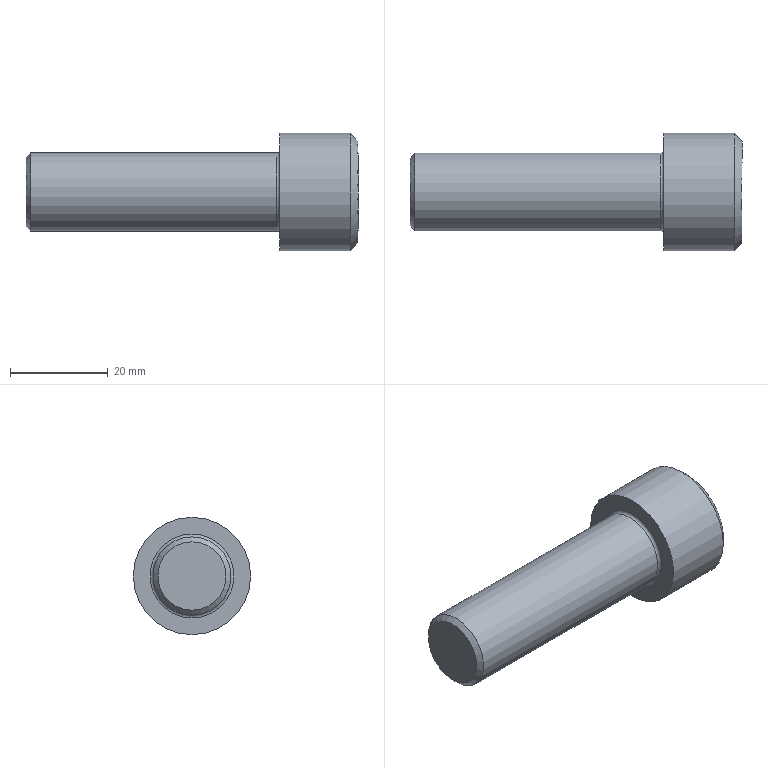Part | STEP file | solid 73 | 1 solid | 21 faces | box 68 x 24 x 24 mm | volume 16217 mm3 | plane 10 | sphere 6 | cylinder 2 | cone 2 | torus 1 | commonest cylinder face diameters 16 x1 24 x1